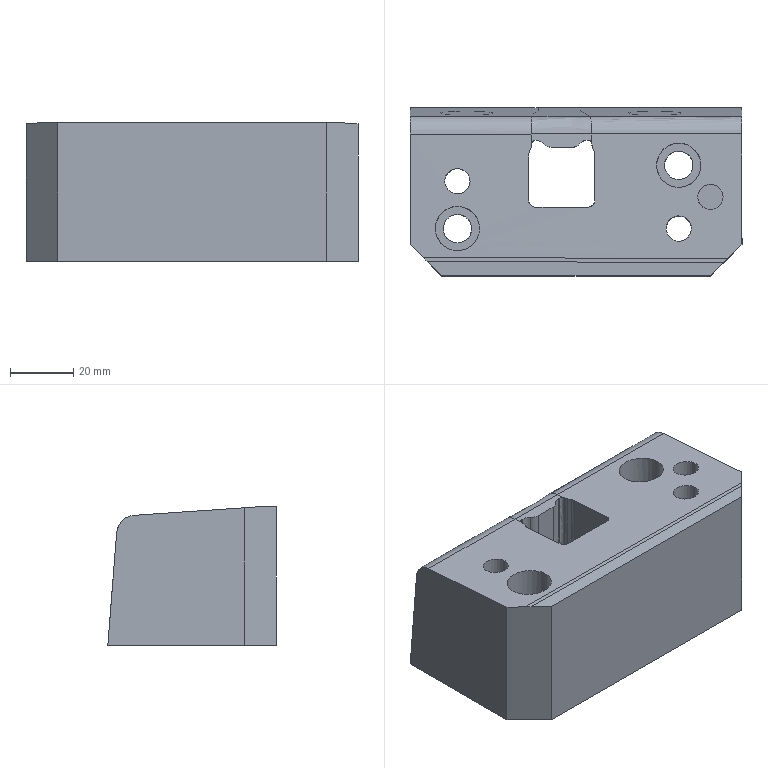Part | NX | features solid 2 | 1 solid | 56 faces | box 105 x 53.264 x 43.898 mm | volume 190464 mm3 | spline 30 | plane 20 | cylinder 6 | commonest cylinder face diameters 8 x3 9 x2 32 x1